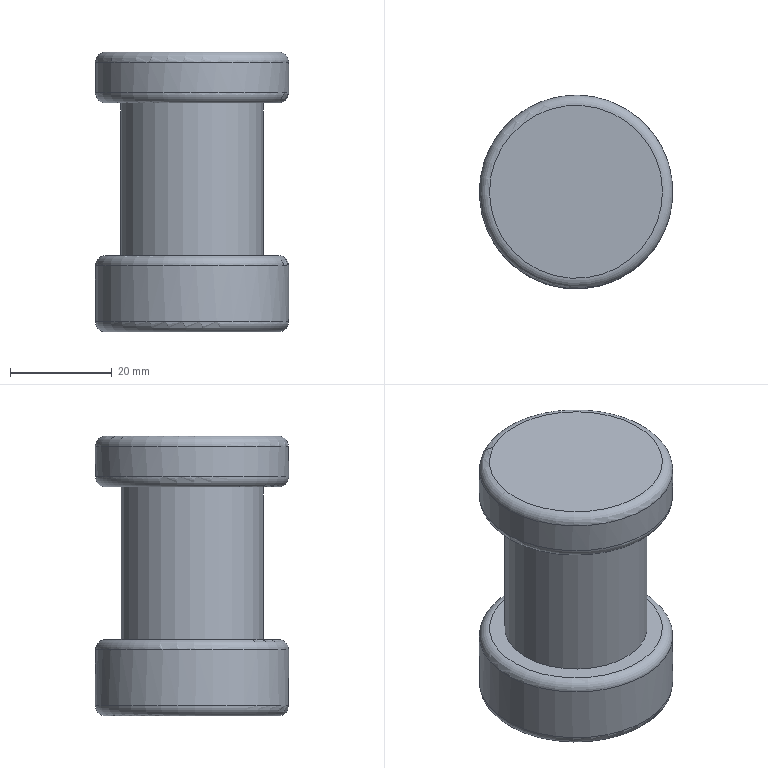Part | NX | features solid 2 | 1 solid | 15 faces | box 38 x 38 x 55 mm | volume 42552 mm3 | cylinder 5 | plane 4 | torus 4 | cone 2 | commonest cylinder face diameters 38 x2 12 x1 18 x1 28 x1
STEP:
#1=CARTESIAN_POINT('',(-212.449,-367.722,141.18));
#2=VERTEX_POINT('',#1);
#3=CARTESIAN_POINT('',(-230.,-375.,141.18));
#4=DIRECTION('',(0.,0.,1.));
#5=DIRECTION('',(0.9237,0.383,0.));
#6=AXIS2_PLACEMENT_3D('',#3,#4,#5);
#7=CIRCLE('',#6,19.);
#8=EDGE_CURVE('',#2,#2,#7,.F.);
#9=ORIENTED_EDGE('',*,*,#8,.T.);
#10=EDGE_LOOP('',(#9));
#11=FACE_BOUND('',#10,.T.);
#12=CARTESIAN_POINT('',(-247.551,-382.278,130.18));
#13=VERTEX_POINT('',#12);
#14=CARTESIAN_POINT('',(-230.,-375.,130.18));
#15=DIRECTION('',(0.,0.,-1.));
#16=DIRECTION('',(-0.9237,-0.383,0.));
#17=AXIS2_PLACEMENT_3D('',#14,#15,#16);
#18=CIRCLE('',#17,19.);
#19=EDGE_CURVE('',#13,#13,#18,.F.);
#20=ORIENTED_EDGE('',*,*,#19,.T.);
#21=EDGE_LOOP('',(#20));
#22=FACE_BOUND('',#21,.T.);
#23=CARTESIAN_POINT('',(-230.,-375.,161.517));
#24=DIRECTION('',(0.,0.,-1.));
#25=DIRECTION('',(-0.9237,-0.383,0.));
#26=AXIS2_PLACEMENT_3D('',#23,#24,#25);
#27=CYLINDRICAL_SURFACE('',#26,19.);
#28=ADVANCED_FACE('',(#11,#22),#27,.T.);
#29=CARTESIAN_POINT('',(-221.686,-371.553,128.18));
#30=VERTEX_POINT('',#29);
#31=CARTESIAN_POINT('',(-230.,-375.,128.18));
#32=DIRECTION('',(0.,0.,1.));
#33=DIRECTION('',(0.9237,0.383,0.));
#34=AXIS2_PLACEMENT_3D('',#31,#32,#33);
#35=CIRCLE('',#34,9.);
#36=EDGE_CURVE('',#30,#30,#35,.T.);
#37=ORIENTED_EDGE('',*,*,#36,.T.);
#38=EDGE_LOOP('',(#37));
#39=FACE_BOUND('',#38,.T.);
#40=CARTESIAN_POINT('',(-245.703,-381.512,128.18));
#41=VERTEX_POINT('',#40);
#42=CARTESIAN_POINT('',(-230.,-375.,128.18));
#43=DIRECTION('',(0.,0.,-1.));
#44=DIRECTION('',(-0.9237,-0.383,0.));
#45=AXIS2_PLACEMENT_3D('',#42,#43,#44);
#46=CIRCLE('',#45,17.);
#47=EDGE_CURVE('',#41,#41,#46,.T.);
#48=ORIENTED_EDGE('',*,*,#47,.T.);
#49=EDGE_LOOP('',(#48));
#50=FACE_BOUND('',#49,.T.);
#51=CARTESIAN_POINT('',(-230.,-375.,128.18));
#52=DIRECTION('',(0.,0.,-1.));
#53=DIRECTION('',(-0.9237,-0.383,0.));
#54=AXIS2_PLACEMENT_3D('',#51,#52,#53);
#55=PLANE('',#54);
#56=ADVANCED_FACE('',(#39,#50),#55,.T.);
#57=CARTESIAN_POINT('',(-214.297,-368.488,143.18));
#58=VERTEX_POINT('',#57);
#59=CARTESIAN_POINT('',(-230.,-375.,143.18));
#60=DIRECTION('',(0.,0.,1.));
#61=DIRECTION('',(0.9237,0.383,0.));
#62=AXIS2_PLACEMENT_3D('',#59,#60,#61);
#63=CIRCLE('',#62,17.);
#64=EDGE_CURVE('',#58,#58,#63,.T.);
#65=ORIENTED_EDGE('',*,*,#64,.T.);
#66=EDGE_LOOP('',(#65));
#67=FACE_BOUND('',#66,.T.);
#68=CARTESIAN_POINT('',(-242.932,-380.363,143.18));
#69=VERTEX_POINT('',#68);
#70=CARTESIAN_POINT('',(-230.,-375.,143.18));
#71=DIRECTION('',(0.,0.,-1.));
#72=DIRECTION('',(-0.9237,-0.383,0.));
#73=AXIS2_PLACEMENT_3D('',#70,#71,#72);
#74=CIRCLE('',#73,14.);
#75=EDGE_CURVE('',#69,#69,#74,.T.);
#76=ORIENTED_EDGE('',*,*,#75,.T.);
#77=EDGE_LOOP('',(#76));
#78=FACE_BOUND('',#77,.T.);
#79=CARTESIAN_POINT('',(-230.,-375.,143.18));
#80=DIRECTION('',(0.,0.,1.));
#81=DIRECTION('',(0.9237,0.383,0.));
#82=AXIS2_PLACEMENT_3D('',#79,#80,#81);
#83=PLANE('',#82);
#84=ADVANCED_FACE('',(#67,#78),#83,.T.);
#85=CARTESIAN_POINT('',(-214.297,-368.488,173.18));
#86=VERTEX_POINT('',#85);
#87=CARTESIAN_POINT('',(-230.,-375.,173.18));
#88=DIRECTION('',(0.,0.,1.));
#89=DIRECTION('',(0.9237,0.383,0.));
#90=AXIS2_PLACEMENT_3D('',#87,#88,#89);
#91=CIRCLE('',#90,17.);
#92=EDGE_CURVE('',#86,#86,#91,.F.);
#93=ORIENTED_EDGE('',*,*,#92,.T.);
#94=EDGE_LOOP('',(#93));
#95=FACE_BOUND('',#94,.T.);
#96=CARTESIAN_POINT('',(-242.932,-380.363,173.18));
#97=VERTEX_POINT('',#96);
#98=CARTESIAN_POINT('',(-230.,-375.,173.18));
#99=DIRECTION('',(0.,0.,-1.));
#100=DIRECTION('',(-0.9237,-0.383,0.));
#101=AXIS2_PLACEMENT_3D('',#98,#99,#100);
#102=CIRCLE('',#101,14.);
#103=EDGE_CURVE('',#97,#97,#102,.T.);
#104=ORIENTED_EDGE('',*,*,#103,.F.);
#105=EDGE_LOOP('',(#104));
#106=FACE_BOUND('',#105,.T.);
#107=CARTESIAN_POINT('',(-230.,-375.,173.18));
#108=DIRECTION('',(0.,0.,1.));
#109=DIRECTION('',(0.9237,0.383,0.));
#110=AXIS2_PLACEMENT_3D('',#107,#108,#109);
#111=PLANE('',#110);
#112=ADVANCED_FACE('',(#95,#106),#111,.F.);
#113=ORIENTED_EDGE('',*,*,#75,.F.);
#114=EDGE_LOOP('',(#113));
#115=FACE_BOUND('',#114,.T.);
#116=ORIENTED_EDGE('',*,*,#103,.T.);
#117=EDGE_LOOP('',(#116));
#118=FACE_BOUND('',#117,.T.);
#119=CARTESIAN_POINT('',(-230.,-375.,173.18));
#120=DIRECTION('',(0.,0.,-1.));
#121=DIRECTION('',(-0.9237,-0.383,0.));
#122=AXIS2_PLACEMENT_3D('',#119,#120,#121);
#123=CYLINDRICAL_SURFACE('',#122,14.);
#124=ADVANCED_FACE('',(#115,#118),#123,.T.);
#125=CARTESIAN_POINT('',(-245.703,-381.512,183.18));
#126=VERTEX_POINT('',#125);
#127=CARTESIAN_POINT('',(-230.,-375.,183.18));
#128=DIRECTION('',(0.,0.,-1.));
#129=DIRECTION('',(-0.9237,-0.383,0.));
#130=AXIS2_PLACEMENT_3D('',#127,#128,#129);
#131=CIRCLE('',#130,17.);
#132=EDGE_CURVE('',#126,#126,#131,.F.);
#133=ORIENTED_EDGE('',*,*,#132,.T.);
#134=EDGE_LOOP('',(#133));
#135=FACE_BOUND('',#134,.T.);
#136=CARTESIAN_POINT('',(-230.,-375.,183.18));
#137=DIRECTION('',(0.,0.,-1.));
#138=DIRECTION('',(-0.9237,-0.383,0.));
#139=AXIS2_PLACEMENT_3D('',#136,#137,#138);
#140=PLANE('',#139);
#141=ADVANCED_FACE('',(#135),#140,.F.);
#142=CARTESIAN_POINT('',(-247.551,-382.278,181.18));
#143=VERTEX_POINT('',#142);
#144=CARTESIAN_POINT('',(-230.,-375.,181.18));
#145=DIRECTION('',(0.,0.,-1.));
#146=DIRECTION('',(-0.9237,-0.383,0.));
#147=AXIS2_PLACEMENT_3D('',#144,#145,#146);
#148=CIRCLE('',#147,19.);
#149=EDGE_CURVE('',#143,#143,#148,.T.);
#150=ORIENTED_EDGE('',*,*,#149,.T.);
#151=EDGE_LOOP('',(#150));
#152=FACE_BOUND('',#151,.T.);
#153=CARTESIAN_POINT('',(-212.449,-367.722,175.18));
#154=VERTEX_POINT('',#153);
#155=CARTESIAN_POINT('',(-230.,-375.,175.18));
#156=DIRECTION('',(0.,0.,1.));
#157=DIRECTION('',(0.9237,0.383,0.));
#158=AXIS2_PLACEMENT_3D('',#155,#156,#157);
#159=CIRCLE('',#158,19.);
#160=EDGE_CURVE('',#154,#154,#159,.T.);
#161=ORIENTED_EDGE('',*,*,#160,.T.);
#162=EDGE_LOOP('',(#161));
#163=FACE_BOUND('',#162,.T.);
#164=CARTESIAN_POINT('',(-230.,-375.,161.517));
#165=DIRECTION('',(0.,0.,-1.));
#166=DIRECTION('',(-0.9237,-0.383,0.));
#167=AXIS2_PLACEMENT_3D('',#164,#165,#166);
#168=CYLINDRICAL_SURFACE('',#167,19.);
#169=ADVANCED_FACE('',(#152,#163),#168,.T.);
#170=ORIENTED_EDGE('',*,*,#64,.F.);
#171=EDGE_LOOP('',(#170));
#172=FACE_BOUND('',#171,.T.);
#173=ORIENTED_EDGE('',*,*,#8,.F.);
#174=EDGE_LOOP('',(#173));
#175=FACE_BOUND('',#174,.T.);
#176=CARTESIAN_POINT('',(-230.,-375.,141.18));
#177=DIRECTION('',(0.,0.,1.));
#178=DIRECTION('',(0.9237,0.383,0.));
#179=AXIS2_PLACEMENT_3D('',#176,#177,#178);
#180=TOROIDAL_SURFACE('',#179,17.,2.);
#181=ADVANCED_FACE('',(#172,#175),#180,.T.);
#182=ORIENTED_EDGE('',*,*,#19,.F.);
#183=EDGE_LOOP('',(#182));
#184=FACE_BOUND('',#183,.T.);
#185=ORIENTED_EDGE('',*,*,#47,.F.);
#186=EDGE_LOOP('',(#185));
#187=FACE_BOUND('',#186,.T.);
#188=CARTESIAN_POINT('',(-230.,-375.,130.18));
#189=DIRECTION('',(0.,0.,-1.));
#190=DIRECTION('',(-0.9237,-0.383,0.));
#191=AXIS2_PLACEMENT_3D('',#188,#189,#190);
#192=TOROIDAL_SURFACE('',#191,17.,2.);
#193=ADVANCED_FACE('',(#184,#187),#192,.T.);
#194=ORIENTED_EDGE('',*,*,#132,.F.);
#195=EDGE_LOOP('',(#194));
#196=FACE_BOUND('',#195,.T.);
#197=ORIENTED_EDGE('',*,*,#149,.F.);
#198=EDGE_LOOP('',(#197));
#199=FACE_BOUND('',#198,.T.);
#200=CARTESIAN_POINT('',(-230.,-375.,181.18));
#201=DIRECTION('',(0.,0.,-1.));
#202=DIRECTION('',(-0.9237,-0.383,0.));
#203=AXIS2_PLACEMENT_3D('',#200,#201,#202);
#204=TOROIDAL_SURFACE('',#203,17.,2.);
#205=ADVANCED_FACE('',(#196,#199),#204,.T.);
#206=ORIENTED_EDGE('',*,*,#92,.F.);
#207=EDGE_LOOP('',(#206));
#208=FACE_BOUND('',#207,.T.);
#209=ORIENTED_EDGE('',*,*,#160,.F.);
#210=EDGE_LOOP('',(#209));
#211=FACE_BOUND('',#210,.T.);
#212=CARTESIAN_POINT('',(-230.,-375.,175.18));
#213=DIRECTION('',(0.,0.,1.));
#214=DIRECTION('',(0.9237,0.383,0.));
#215=AXIS2_PLACEMENT_3D('',#212,#213,#214);
#216=TOROIDAL_SURFACE('',#215,17.,2.);
#217=ADVANCED_FACE('',(#208,#211),#216,.T.);
#218=CARTESIAN_POINT('',(-221.686,-371.553,128.19));
#219=VERTEX_POINT('',#218);
#220=CARTESIAN_POINT('',(-230.,-375.,128.19));
#221=DIRECTION('',(0.,0.,1.));
#222=DIRECTION('',(0.9237,0.383,0.));
#223=AXIS2_PLACEMENT_3D('',#220,#221,#222);
#224=CIRCLE('',#223,9.);
#225=EDGE_CURVE('',#219,#219,#224,.T.);
#226=ORIENTED_EDGE('',*,*,#225,.F.);
#227=EDGE_LOOP('',(#226));
#228=FACE_BOUND('',#227,.T.);
#229=CARTESIAN_POINT('',(-235.542,-377.298,133.386));
#230=VERTEX_POINT('',#229);
#231=CARTESIAN_POINT('',(-230.,-375.,133.386));
#232=DIRECTION('',(0.,0.,-1.));
#233=DIRECTION('',(-0.9237,-0.383,0.));
#234=AXIS2_PLACEMENT_3D('',#231,#232,#233);
#235=CIRCLE('',#234,6.);
#236=EDGE_CURVE('',#230,#230,#235,.T.);
#237=ORIENTED_EDGE('',*,*,#236,.F.);
#238=EDGE_LOOP('',(#237));
#239=FACE_BOUND('',#238,.T.);
#240=CARTESIAN_POINT('',(-230.,-375.,128.19));
#241=DIRECTION('',(0.,0.,-1.));
#242=DIRECTION('',(-0.9237,-0.383,0.));
#243=AXIS2_PLACEMENT_3D('',#240,#241,#242);
#244=CONICAL_SURFACE('',#243,9.,0.5236);
#245=ADVANCED_FACE('',(#228,#239),#244,.F.);
#246=ORIENTED_EDGE('',*,*,#225,.T.);
#247=EDGE_LOOP('',(#246));
#248=FACE_BOUND('',#247,.T.);
#249=ORIENTED_EDGE('',*,*,#36,.F.);
#250=EDGE_LOOP('',(#249));
#251=FACE_BOUND('',#250,.T.);
#252=CARTESIAN_POINT('',(-230.,-375.,128.18));
#253=DIRECTION('',(0.,0.,1.));
#254=DIRECTION('',(0.9237,0.383,0.));
#255=AXIS2_PLACEMENT_3D('',#252,#253,#254);
#256=CYLINDRICAL_SURFACE('',#255,9.);
#257=ADVANCED_FACE('',(#248,#251),#256,.F.);
#258=CARTESIAN_POINT('',(-224.458,-372.702,158.18));
#259=VERTEX_POINT('',#258);
#260=CARTESIAN_POINT('',(-230.,-375.,158.18));
#261=DIRECTION('',(0.,0.,1.));
#262=DIRECTION('',(0.9237,0.383,0.));
#263=AXIS2_PLACEMENT_3D('',#260,#261,#262);
#264=CIRCLE('',#263,6.);
#265=EDGE_CURVE('',#259,#259,#264,.T.);
#266=ORIENTED_EDGE('',*,*,#265,.F.);
#267=EDGE_LOOP('',(#266));
#268=FACE_BOUND('',#267,.T.);
#269=CARTESIAN_POINT('',(-230.,-375.,161.785));
#270=VERTEX_POINT('',#269);
#271=VERTEX_LOOP('',#270);
#272=FACE_BOUND('',#271,.T.);
#273=CARTESIAN_POINT('',(-230.,-375.,158.18));
#274=DIRECTION('',(0.,0.,-1.));
#275=DIRECTION('',(-0.9237,-0.383,0.));
#276=AXIS2_PLACEMENT_3D('',#273,#274,#275);
#277=CONICAL_SURFACE('',#276,6.,1.03);
#278=ADVANCED_FACE('',(#268,#272),#277,.F.);
#279=ORIENTED_EDGE('',*,*,#236,.T.);
#280=EDGE_LOOP('',(#279));
#281=FACE_BOUND('',#280,.T.);
#282=ORIENTED_EDGE('',*,*,#265,.T.);
#283=EDGE_LOOP('',(#282));
#284=FACE_BOUND('',#283,.T.);
#285=CARTESIAN_POINT('',(-230.,-375.,128.18));
#286=DIRECTION('',(0.,0.,1.));
#287=DIRECTION('',(0.9237,0.383,0.));
#288=AXIS2_PLACEMENT_3D('',#285,#286,#287);
#289=CYLINDRICAL_SURFACE('',#288,6.);
#290=ADVANCED_FACE('',(#281,#284),#289,.F.);
#291=CLOSED_SHELL('',(#28,#56,#84,#112,#124,#141,#169,#181,#193,#205,#217,#245,#257,#278,#290));
#292=MANIFOLD_SOLID_BREP('',#291);
#293=(LENGTH_UNIT()NAMED_UNIT(*)SI_UNIT(.MILLI.,.METRE.));
#294=UNCERTAINTY_MEASURE_WITH_UNIT(LENGTH_MEASURE(0.00001),#293,'','');
#295=(NAMED_UNIT(*)PLANE_ANGLE_UNIT()SI_UNIT($,.RADIAN.));
#296=(NAMED_UNIT(*)SI_UNIT($,.STERADIAN.)SOLID_ANGLE_UNIT());
#297=(GEOMETRIC_REPRESENTATION_CONTEXT(3)GLOBAL_UNCERTAINTY_ASSIGNED_CONTEXT((#294))GLOBAL_UNIT_ASSIGNED_CONTEXT((#293,#295,#296))REPRESENTATION_CONTEXT('',''));
#298=ADVANCED_BREP_SHAPE_REPRESENTATION('',(#292),#297);